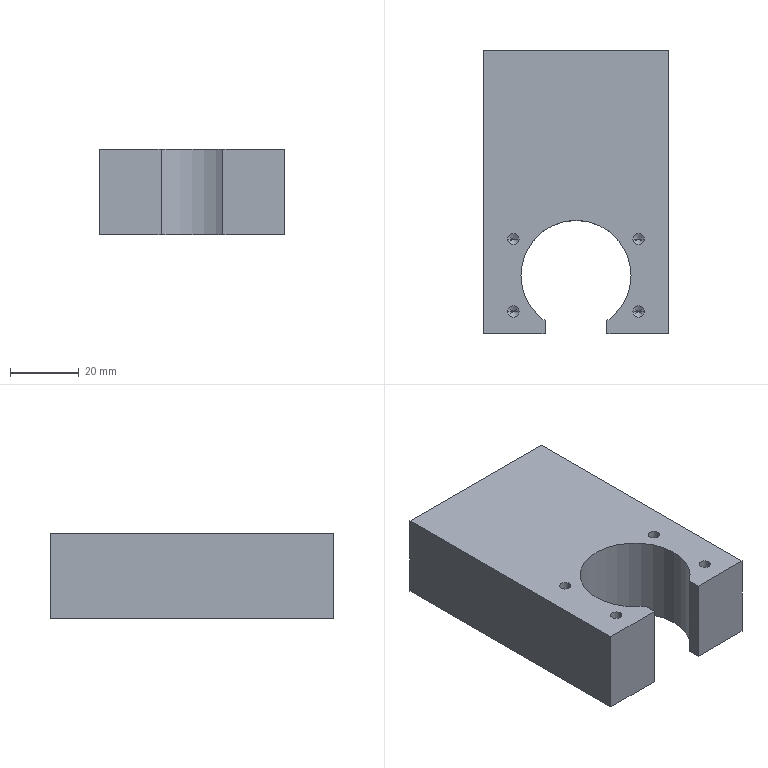Part | SolidWorks | features HoleWzd 2, 3DProfileFeature 1, Extrusion 1 | 1 solid | 52 faces | box 54 x 82.5 x 25 mm | volume 89091 mm3 | cone 24 | cylinder 19 | plane 9 | commonest cylinder face diameters 3.3 x8 5 x8 32 x3
STEP:
#1=CARTESIAN_POINT('',(-20.,64.975,3.));
#2=VERTEX_POINT('',#1);
#3=CARTESIAN_POINT('',(-20.,64.975,8.));
#4=VERTEX_POINT('',#3);
#5=CARTESIAN_POINT('',(-20.,64.975,5.5));
#6=DIRECTION('',(0.,1.,0.));
#7=DIRECTION('',(0.,0.,1.));
#8=AXIS2_PLACEMENT_3D('',#5,#6,#7);
#9=CIRCLE('',#8,2.5);
#10=EDGE_CURVE('',#2,#4,#9,.T.);
#11=ORIENTED_EDGE('',*,*,#10,.F.);
#12=CARTESIAN_POINT('',(-20.,65.5,2.475));
#13=VERTEX_POINT('',#12);
#14=CARTESIAN_POINT('',(-20.,65.5,2.475));
#15=DIRECTION('',(0.,0.7071,-0.7071));
#16=VECTOR('',#15,1000.);
#17=LINE('',#14,#16);
#18=EDGE_CURVE('',#2,#13,#17,.T.);
#19=ORIENTED_EDGE('',*,*,#18,.T.);
#20=CARTESIAN_POINT('',(-20.,65.5,8.525));
#21=VERTEX_POINT('',#20);
#22=CARTESIAN_POINT('',(-20.,65.5,5.5));
#23=DIRECTION('',(0.,1.,0.));
#24=DIRECTION('',(0.,0.,1.));
#25=AXIS2_PLACEMENT_3D('',#22,#23,#24);
#26=CIRCLE('',#25,3.025);
#27=EDGE_CURVE('',#13,#21,#26,.T.);
#28=ORIENTED_EDGE('',*,*,#27,.T.);
#29=CARTESIAN_POINT('',(-20.,65.5,8.525));
#30=DIRECTION('',(0.,0.7071,0.7071));
#31=VECTOR('',#30,1000.);
#32=LINE('',#29,#31);
#33=EDGE_CURVE('',#4,#21,#32,.T.);
#34=ORIENTED_EDGE('',*,*,#33,.F.);
#35=EDGE_LOOP('',(#11,#19,#28,#34));
#36=FACE_OUTER_BOUND('',#35,.T.);
#37=CARTESIAN_POINT('',(-20.,65.5,5.5));
#38=DIRECTION('',(0.,1.,0.));
#39=DIRECTION('',(0.,0.,1.));
#40=AXIS2_PLACEMENT_3D('',#37,#38,#39);
#41=CONICAL_SURFACE('',#40,3.025,0.7854);
#42=ADVANCED_FACE('',(#36),#41,.F.);
#43=CARTESIAN_POINT('',(-20.,53.5,3.));
#44=VERTEX_POINT('',#43);
#45=CARTESIAN_POINT('',(-20.,53.5,8.));
#46=VERTEX_POINT('',#45);
#47=CARTESIAN_POINT('',(-20.,53.5,5.5));
#48=DIRECTION('',(0.,1.,0.));
#49=DIRECTION('',(0.,0.,1.));
#50=AXIS2_PLACEMENT_3D('',#47,#48,#49);
#51=CIRCLE('',#50,2.5);
#52=EDGE_CURVE('',#44,#46,#51,.T.);
#53=ORIENTED_EDGE('',*,*,#52,.F.);
#54=CARTESIAN_POINT('',(-20.,65.5,3.));
#55=DIRECTION('',(0.,1.,0.));
#56=VECTOR('',#55,1000.);
#57=LINE('',#54,#56);
#58=EDGE_CURVE('',#44,#2,#57,.T.);
#59=ORIENTED_EDGE('',*,*,#58,.T.);
#60=ORIENTED_EDGE('',*,*,#10,.T.);
#61=CARTESIAN_POINT('',(-20.,65.5,8.));
#62=DIRECTION('',(0.,1.,0.));
#63=VECTOR('',#62,1000.);
#64=LINE('',#61,#63);
#65=EDGE_CURVE('',#46,#4,#64,.T.);
#66=ORIENTED_EDGE('',*,*,#65,.F.);
#67=EDGE_LOOP('',(#53,#59,#60,#66));
#68=FACE_OUTER_BOUND('',#67,.T.);
#69=CARTESIAN_POINT('',(-20.,65.5,5.5));
#70=DIRECTION('',(0.,1.,0.));
#71=DIRECTION('',(0.,0.,1.));
#72=AXIS2_PLACEMENT_3D('',#69,#70,#71);
#73=CYLINDRICAL_SURFACE('',#72,2.5);
#74=ADVANCED_FACE('',(#68),#73,.F.);
#75=CARTESIAN_POINT('',(-20.,51.998,5.5));
#76=VERTEX_POINT('',#75);
#77=CARTESIAN_POINT('',(-20.,53.5,8.));
#78=DIRECTION('',(0.,0.515,0.8572));
#79=VECTOR('',#78,1000.);
#80=LINE('',#77,#79);
#81=EDGE_CURVE('',#76,#46,#80,.T.);
#82=ORIENTED_EDGE('',*,*,#81,.F.);
#83=CARTESIAN_POINT('',(-20.,53.5,3.));
#84=DIRECTION('',(0.,0.515,-0.8572));
#85=VECTOR('',#84,1000.);
#86=LINE('',#83,#85);
#87=EDGE_CURVE('',#76,#44,#86,.T.);
#88=ORIENTED_EDGE('',*,*,#87,.T.);
#89=ORIENTED_EDGE('',*,*,#52,.T.);
#90=EDGE_LOOP('',(#82,#88,#89));
#91=FACE_OUTER_BOUND('',#90,.T.);
#92=CARTESIAN_POINT('',(-20.,53.5,5.5));
#93=DIRECTION('',(0.,1.,0.));
#94=DIRECTION('',(0.,0.,1.));
#95=AXIS2_PLACEMENT_3D('',#92,#93,#94);
#96=CONICAL_SURFACE('',#95,2.5,1.03);
#97=ADVANCED_FACE('',(#91),#96,.F.);
#98=CARTESIAN_POINT('',(-20.,64.975,-8.));
#99=VERTEX_POINT('',#98);
#100=CARTESIAN_POINT('',(-20.,64.975,-3.));
#101=VERTEX_POINT('',#100);
#102=CARTESIAN_POINT('',(-20.,64.975,-5.5));
#103=DIRECTION('',(0.,1.,0.));
#104=DIRECTION('',(0.,0.,1.));
#105=AXIS2_PLACEMENT_3D('',#102,#103,#104);
#106=CIRCLE('',#105,2.5);
#107=EDGE_CURVE('',#99,#101,#106,.T.);
#108=ORIENTED_EDGE('',*,*,#107,.F.);
#109=CARTESIAN_POINT('',(-20.,65.5,-8.525));
#110=VERTEX_POINT('',#109);
#111=CARTESIAN_POINT('',(-20.,65.5,-8.525));
#112=DIRECTION('',(0.,0.7071,-0.7071));
#113=VECTOR('',#112,1000.);
#114=LINE('',#111,#113);
#115=EDGE_CURVE('',#99,#110,#114,.T.);
#116=ORIENTED_EDGE('',*,*,#115,.T.);
#117=CARTESIAN_POINT('',(-20.,65.5,-2.475));
#118=VERTEX_POINT('',#117);
#119=CARTESIAN_POINT('',(-20.,65.5,-5.5));
#120=DIRECTION('',(0.,1.,0.));
#121=DIRECTION('',(0.,0.,1.));
#122=AXIS2_PLACEMENT_3D('',#119,#120,#121);
#123=CIRCLE('',#122,3.025);
#124=EDGE_CURVE('',#110,#118,#123,.T.);
#125=ORIENTED_EDGE('',*,*,#124,.T.);
#126=CARTESIAN_POINT('',(-20.,65.5,-2.475));
#127=DIRECTION('',(0.,0.7071,0.7071));
#128=VECTOR('',#127,1000.);
#129=LINE('',#126,#128);
#130=EDGE_CURVE('',#101,#118,#129,.T.);
#131=ORIENTED_EDGE('',*,*,#130,.F.);
#132=EDGE_LOOP('',(#108,#116,#125,#131));
#133=FACE_OUTER_BOUND('',#132,.T.);
#134=CARTESIAN_POINT('',(-20.,65.5,-5.5));
#135=DIRECTION('',(0.,1.,0.));
#136=DIRECTION('',(0.,0.,1.));
#137=AXIS2_PLACEMENT_3D('',#134,#135,#136);
#138=CONICAL_SURFACE('',#137,3.025,0.7854);
#139=ADVANCED_FACE('',(#133),#138,.F.);
#140=CARTESIAN_POINT('',(-20.,53.5,-8.));
#141=VERTEX_POINT('',#140);
#142=CARTESIAN_POINT('',(-20.,53.5,-3.));
#143=VERTEX_POINT('',#142);
#144=CARTESIAN_POINT('',(-20.,53.5,-5.5));
#145=DIRECTION('',(0.,1.,0.));
#146=DIRECTION('',(0.,0.,1.));
#147=AXIS2_PLACEMENT_3D('',#144,#145,#146);
#148=CIRCLE('',#147,2.5);
#149=EDGE_CURVE('',#141,#143,#148,.T.);
#150=ORIENTED_EDGE('',*,*,#149,.F.);
#151=CARTESIAN_POINT('',(-20.,65.5,-8.));
#152=DIRECTION('',(0.,1.,0.));
#153=VECTOR('',#152,1000.);
#154=LINE('',#151,#153);
#155=EDGE_CURVE('',#141,#99,#154,.T.);
#156=ORIENTED_EDGE('',*,*,#155,.T.);
#157=ORIENTED_EDGE('',*,*,#107,.T.);
#158=CARTESIAN_POINT('',(-20.,65.5,-3.));
#159=DIRECTION('',(0.,1.,0.));
#160=VECTOR('',#159,1000.);
#161=LINE('',#158,#160);
#162=EDGE_CURVE('',#143,#101,#161,.T.);
#163=ORIENTED_EDGE('',*,*,#162,.F.);
#164=EDGE_LOOP('',(#150,#156,#157,#163));
#165=FACE_OUTER_BOUND('',#164,.T.);
#166=CARTESIAN_POINT('',(-20.,65.5,-5.5));
#167=DIRECTION('',(0.,1.,0.));
#168=DIRECTION('',(0.,0.,1.));
#169=AXIS2_PLACEMENT_3D('',#166,#167,#168);
#170=CYLINDRICAL_SURFACE('',#169,2.5);
#171=ADVANCED_FACE('',(#165),#170,.F.);
#172=CARTESIAN_POINT('',(-20.,51.998,-5.5));
#173=VERTEX_POINT('',#172);
#174=CARTESIAN_POINT('',(-20.,53.5,-3.));
#175=DIRECTION('',(0.,0.515,0.8572));
#176=VECTOR('',#175,1000.);
#177=LINE('',#174,#176);
#178=EDGE_CURVE('',#173,#143,#177,.T.);
#179=ORIENTED_EDGE('',*,*,#178,.F.);
#180=CARTESIAN_POINT('',(-20.,53.5,-8.));
#181=DIRECTION('',(0.,0.515,-0.8572));
#182=VECTOR('',#181,1000.);
#183=LINE('',#180,#182);
#184=EDGE_CURVE('',#173,#141,#183,.T.);
#185=ORIENTED_EDGE('',*,*,#184,.T.);
#186=ORIENTED_EDGE('',*,*,#149,.T.);
#187=EDGE_LOOP('',(#179,#185,#186));
#188=FACE_OUTER_BOUND('',#187,.T.);
#189=CARTESIAN_POINT('',(-20.,53.5,-5.5));
#190=DIRECTION('',(0.,1.,0.));
#191=DIRECTION('',(0.,0.,1.));
#192=AXIS2_PLACEMENT_3D('',#189,#190,#191);
#193=CONICAL_SURFACE('',#192,2.5,1.03);
#194=ADVANCED_FACE('',(#188),#193,.F.);
#195=CARTESIAN_POINT('',(20.,64.975,-8.));
#196=VERTEX_POINT('',#195);
#197=CARTESIAN_POINT('',(20.,64.975,-3.));
#198=VERTEX_POINT('',#197);
#199=CARTESIAN_POINT('',(20.,64.975,-5.5));
#200=DIRECTION('',(0.,1.,0.));
#201=DIRECTION('',(0.,0.,1.));
#202=AXIS2_PLACEMENT_3D('',#199,#200,#201);
#203=CIRCLE('',#202,2.5);
#204=EDGE_CURVE('',#196,#198,#203,.T.);
#205=ORIENTED_EDGE('',*,*,#204,.F.);
#206=CARTESIAN_POINT('',(20.,65.5,-8.525));
#207=VERTEX_POINT('',#206);
#208=CARTESIAN_POINT('',(20.,65.5,-8.525));
#209=DIRECTION('',(0.,0.7071,-0.7071));
#210=VECTOR('',#209,1000.);
#211=LINE('',#208,#210);
#212=EDGE_CURVE('',#196,#207,#211,.T.);
#213=ORIENTED_EDGE('',*,*,#212,.T.);
#214=CARTESIAN_POINT('',(20.,65.5,-2.475));
#215=VERTEX_POINT('',#214);
#216=CARTESIAN_POINT('',(20.,65.5,-5.5));
#217=DIRECTION('',(0.,1.,0.));
#218=DIRECTION('',(0.,0.,1.));
#219=AXIS2_PLACEMENT_3D('',#216,#217,#218);
#220=CIRCLE('',#219,3.025);
#221=EDGE_CURVE('',#207,#215,#220,.T.);
#222=ORIENTED_EDGE('',*,*,#221,.T.);
#223=CARTESIAN_POINT('',(20.,65.5,-2.475));
#224=DIRECTION('',(0.,0.7071,0.7071));
#225=VECTOR('',#224,1000.);
#226=LINE('',#223,#225);
#227=EDGE_CURVE('',#198,#215,#226,.T.);
#228=ORIENTED_EDGE('',*,*,#227,.F.);
#229=EDGE_LOOP('',(#205,#213,#222,#228));
#230=FACE_OUTER_BOUND('',#229,.T.);
#231=CARTESIAN_POINT('',(20.,65.5,-5.5));
#232=DIRECTION('',(0.,1.,0.));
#233=DIRECTION('',(0.,0.,1.));
#234=AXIS2_PLACEMENT_3D('',#231,#232,#233);
#235=CONICAL_SURFACE('',#234,3.025,0.7854);
#236=ADVANCED_FACE('',(#230),#235,.F.);
#237=CARTESIAN_POINT('',(20.,53.5,-8.));
#238=VERTEX_POINT('',#237);
#239=CARTESIAN_POINT('',(20.,53.5,-3.));
#240=VERTEX_POINT('',#239);
#241=CARTESIAN_POINT('',(20.,53.5,-5.5));
#242=DIRECTION('',(0.,1.,0.));
#243=DIRECTION('',(0.,0.,1.));
#244=AXIS2_PLACEMENT_3D('',#241,#242,#243);
#245=CIRCLE('',#244,2.5);
#246=EDGE_CURVE('',#238,#240,#245,.T.);
#247=ORIENTED_EDGE('',*,*,#246,.F.);
#248=CARTESIAN_POINT('',(20.,65.5,-8.));
#249=DIRECTION('',(0.,1.,0.));
#250=VECTOR('',#249,1000.);
#251=LINE('',#248,#250);
#252=EDGE_CURVE('',#238,#196,#251,.T.);
#253=ORIENTED_EDGE('',*,*,#252,.T.);
#254=ORIENTED_EDGE('',*,*,#204,.T.);
#255=CARTESIAN_POINT('',(20.,65.5,-3.));
#256=DIRECTION('',(0.,1.,0.));
#257=VECTOR('',#256,1000.);
#258=LINE('',#255,#257);
#259=EDGE_CURVE('',#240,#198,#258,.T.);
#260=ORIENTED_EDGE('',*,*,#259,.F.);
#261=EDGE_LOOP('',(#247,#253,#254,#260));
#262=FACE_OUTER_BOUND('',#261,.T.);
#263=CARTESIAN_POINT('',(20.,65.5,-5.5));
#264=DIRECTION('',(0.,1.,0.));
#265=DIRECTION('',(0.,0.,1.));
#266=AXIS2_PLACEMENT_3D('',#263,#264,#265);
#267=CYLINDRICAL_SURFACE('',#266,2.5);
#268=ADVANCED_FACE('',(#262),#267,.F.);
#269=CARTESIAN_POINT('',(20.,51.998,-5.5));
#270=VERTEX_POINT('',#269);
#271=CARTESIAN_POINT('',(20.,53.5,-3.));
#272=DIRECTION('',(0.,0.515,0.8572));
#273=VECTOR('',#272,1000.);
#274=LINE('',#271,#273);
#275=EDGE_CURVE('',#270,#240,#274,.T.);
#276=ORIENTED_EDGE('',*,*,#275,.F.);
#277=CARTESIAN_POINT('',(20.,53.5,-8.));
#278=DIRECTION('',(0.,0.515,-0.8572));
#279=VECTOR('',#278,1000.);
#280=LINE('',#277,#279);
#281=EDGE_CURVE('',#270,#238,#280,.T.);
#282=ORIENTED_EDGE('',*,*,#281,.T.);
#283=ORIENTED_EDGE('',*,*,#246,.T.);
#284=EDGE_LOOP('',(#276,#282,#283));
#285=FACE_OUTER_BOUND('',#284,.T.);
#286=CARTESIAN_POINT('',(20.,53.5,-5.5));
#287=DIRECTION('',(0.,1.,0.));
#288=DIRECTION('',(0.,0.,1.));
#289=AXIS2_PLACEMENT_3D('',#286,#287,#288);
#290=CONICAL_SURFACE('',#289,2.5,1.03);
#291=ADVANCED_FACE('',(#285),#290,.F.);
#292=CARTESIAN_POINT('',(20.,64.975,3.));
#293=VERTEX_POINT('',#292);
#294=CARTESIAN_POINT('',(20.,64.975,8.));
#295=VERTEX_POINT('',#294);
#296=CARTESIAN_POINT('',(20.,64.975,5.5));
#297=DIRECTION('',(0.,1.,0.));
#298=DIRECTION('',(0.,0.,1.));
#299=AXIS2_PLACEMENT_3D('',#296,#297,#298);
#300=CIRCLE('',#299,2.5);
#301=EDGE_CURVE('',#293,#295,#300,.T.);
#302=ORIENTED_EDGE('',*,*,#301,.F.);
#303=CARTESIAN_POINT('',(20.,65.5,2.475));
#304=VERTEX_POINT('',#303);
#305=CARTESIAN_POINT('',(20.,65.5,2.475));
#306=DIRECTION('',(0.,0.7071,-0.7071));
#307=VECTOR('',#306,1000.);
#308=LINE('',#305,#307);
#309=EDGE_CURVE('',#293,#304,#308,.T.);
#310=ORIENTED_EDGE('',*,*,#309,.T.);
#311=CARTESIAN_POINT('',(20.,65.5,8.525));
#312=VERTEX_POINT('',#311);
#313=CARTESIAN_POINT('',(20.,65.5,5.5));
#314=DIRECTION('',(0.,1.,0.));
#315=DIRECTION('',(0.,0.,1.));
#316=AXIS2_PLACEMENT_3D('',#313,#314,#315);
#317=CIRCLE('',#316,3.025);
#318=EDGE_CURVE('',#304,#312,#317,.T.);
#319=ORIENTED_EDGE('',*,*,#318,.T.);
#320=CARTESIAN_POINT('',(20.,65.5,8.525));
#321=DIRECTION('',(0.,0.7071,0.7071));
#322=VECTOR('',#321,1000.);
#323=LINE('',#320,#322);
#324=EDGE_CURVE('',#295,#312,#323,.T.);
#325=ORIENTED_EDGE('',*,*,#324,.F.);
#326=EDGE_LOOP('',(#302,#310,#319,#325));
#327=FACE_OUTER_BOUND('',#326,.T.);
#328=CARTESIAN_POINT('',(20.,65.5,5.5));
#329=DIRECTION('',(0.,1.,0.));
#330=DIRECTION('',(0.,0.,1.));
#331=AXIS2_PLACEMENT_3D('',#328,#329,#330);
#332=CONICAL_SURFACE('',#331,3.025,0.7854);
#333=ADVANCED_FACE('',(#327),#332,.F.);
#334=CARTESIAN_POINT('',(20.,53.5,3.));
#335=VERTEX_POINT('',#334);
#336=CARTESIAN_POINT('',(20.,53.5,8.));
#337=VERTEX_POINT('',#336);
#338=CARTESIAN_POINT('',(20.,53.5,5.5));
#339=DIRECTION('',(0.,1.,0.));
#340=DIRECTION('',(0.,0.,1.));
#341=AXIS2_PLACEMENT_3D('',#338,#339,#340);
#342=CIRCLE('',#341,2.5);
#343=EDGE_CURVE('',#335,#337,#342,.T.);
#344=ORIENTED_EDGE('',*,*,#343,.F.);
#345=CARTESIAN_POINT('',(20.,65.5,3.));
#346=DIRECTION('',(0.,1.,0.));
#347=VECTOR('',#346,1000.);
#348=LINE('',#345,#347);
#349=EDGE_CURVE('',#335,#293,#348,.T.);
#350=ORIENTED_EDGE('',*,*,#349,.T.);
#351=ORIENTED_EDGE('',*,*,#301,.T.);
#352=CARTESIAN_POINT('',(20.,65.5,8.));
#353=DIRECTION('',(0.,1.,0.));
#354=VECTOR('',#353,1000.);
#355=LINE('',#352,#354);
#356=EDGE_CURVE('',#337,#295,#355,.T.);
#357=ORIENTED_EDGE('',*,*,#356,.F.);
#358=EDGE_LOOP('',(#344,#350,#351,#357));
#359=FACE_OUTER_BOUND('',#358,.T.);
#360=CARTESIAN_POINT('',(20.,65.5,5.5));
#361=DIRECTION('',(0.,1.,0.));
#362=DIRECTION('',(0.,0.,1.));
#363=AXIS2_PLACEMENT_3D('',#360,#361,#362);
#364=CYLINDRICAL_SURFACE('',#363,2.5);
#365=ADVANCED_FACE('',(#359),#364,.F.);
#366=CARTESIAN_POINT('',(20.,51.998,5.5));
#367=VERTEX_POINT('',#366);
#368=CARTESIAN_POINT('',(20.,53.5,8.));
#369=DIRECTION('',(0.,0.515,0.8572));
#370=VECTOR('',#369,1000.);
#371=LINE('',#368,#370);
#372=EDGE_CURVE('',#367,#337,#371,.T.);
#373=ORIENTED_EDGE('',*,*,#372,.F.);
#374=CARTESIAN_POINT('',(20.,53.5,3.));
#375=DIRECTION('',(0.,0.515,-0.8572));
#376=VECTOR('',#375,1000.);
#377=LINE('',#374,#376);
#378=EDGE_CURVE('',#367,#335,#377,.T.);
#379=ORIENTED_EDGE('',*,*,#378,.T.);
#380=ORIENTED_EDGE('',*,*,#343,.T.);
#381=EDGE_LOOP('',(#373,#379,#380));
#382=FACE_OUTER_BOUND('',#381,.T.);
#383=CARTESIAN_POINT('',(20.,53.5,5.5));
#384=DIRECTION('',(0.,1.,0.));
#385=DIRECTION('',(0.,0.,1.));
#386=AXIS2_PLACEMENT_3D('',#383,#384,#385);
#387=CONICAL_SURFACE('',#386,2.5,1.03);
#388=ADVANCED_FACE('',(#382),#387,.F.);
#389=CARTESIAN_POINT('',(16.537,10.5,3.));
#390=VERTEX_POINT('',#389);
#391=CARTESIAN_POINT('',(19.837,10.5,3.));
#392=VERTEX_POINT('',#391);
#393=CARTESIAN_POINT('',(18.187,10.5,3.));
#394=DIRECTION('',(0.,0.,1.));
#395=DIRECTION('',(1.,0.,0.));
#396=AXIS2_PLACEMENT_3D('',#393,#394,#395);
#397=CIRCLE('',#396,1.65);
#398=EDGE_CURVE('',#390,#392,#397,.T.);
#399=ORIENTED_EDGE('',*,*,#398,.F.);
#400=CARTESIAN_POINT('',(16.537,10.5,12.5));
#401=VERTEX_POINT('',#400);
#402=CARTESIAN_POINT('',(16.537,10.5,12.5));
#403=DIRECTION('',(0.,0.,1.));
#404=VECTOR('',#403,1000.);
#405=LINE('',#402,#404);
#406=EDGE_CURVE('',#390,#401,#405,.T.);
#407=ORIENTED_EDGE('',*,*,#406,.T.);
#408=CARTESIAN_POINT('',(19.837,10.5,12.5));
#409=VERTEX_POINT('',#408);
#410=CARTESIAN_POINT('',(18.187,10.5,12.5));
#411=DIRECTION('',(0.,0.,1.));
#412=DIRECTION('',(1.,0.,0.));
#413=AXIS2_PLACEMENT_3D('',#410,#411,#412);
#414=CIRCLE('',#413,1.65);
#415=EDGE_CURVE('',#401,#409,#414,.T.);
#416=ORIENTED_EDGE('',*,*,#415,.T.);
#417=CARTESIAN_POINT('',(19.837,10.5,12.5));
#418=DIRECTION('',(0.,0.,1.));
#419=VECTOR('',#418,1000.);
#420=LINE('',#417,#419);
#421=EDGE_CURVE('',#392,#409,#420,.T.);
#422=ORIENTED_EDGE('',*,*,#421,.F.);
#423=EDGE_LOOP('',(#399,#407,#416,#422));
#424=FACE_OUTER_BOUND('',#423,.T.);
#425=CARTESIAN_POINT('',(18.187,10.5,12.5));
#426=DIRECTION('',(0.,0.,1.));
#427=DIRECTION('',(1.,0.,0.));
#428=AXIS2_PLACEMENT_3D('',#425,#426,#427);
#429=CYLINDRICAL_SURFACE('',#428,1.65);
#430=ADVANCED_FACE('',(#424),#429,.F.);
#431=CARTESIAN_POINT('',(18.187,10.5,2.009));
#432=VERTEX_POINT('',#431);
#433=CARTESIAN_POINT('',(19.837,10.5,3.));
#434=DIRECTION('',(0.8572,0.,0.515));
#435=VECTOR('',#434,1000.);
#436=LINE('',#433,#435);
#437=EDGE_CURVE('',#432,#392,#436,.T.);
#438=ORIENTED_EDGE('',*,*,#437,.F.);
#439=CARTESIAN_POINT('',(16.537,10.5,3.));
#440=DIRECTION('',(-0.8572,0.,0.515));
#441=VECTOR('',#440,1000.);
#442=LINE('',#439,#441);
#443=EDGE_CURVE('',#432,#390,#442,.T.);
#444=ORIENTED_EDGE('',*,*,#443,.T.);
#445=ORIENTED_EDGE('',*,*,#398,.T.);
#446=EDGE_LOOP('',(#438,#444,#445));
#447=FACE_OUTER_BOUND('',#446,.T.);
#448=CARTESIAN_POINT('',(18.187,10.5,3.));
#449=DIRECTION('',(0.,0.,1.));
#450=DIRECTION('',(1.,0.,0.));
#451=AXIS2_PLACEMENT_3D('',#448,#449,#450);
#452=CONICAL_SURFACE('',#451,1.65,1.03);
#453=ADVANCED_FACE('',(#447),#452,.F.);
#454=CARTESIAN_POINT('',(16.537,-10.5,3.));
#455=VERTEX_POINT('',#454);
#456=CARTESIAN_POINT('',(19.837,-10.5,3.));
#457=VERTEX_POINT('',#456);
#458=CARTESIAN_POINT('',(18.187,-10.5,3.));
#459=DIRECTION('',(0.,0.,1.));
#460=DIRECTION('',(1.,0.,0.));
#461=AXIS2_PLACEMENT_3D('',#458,#459,#460);
#462=CIRCLE('',#461,1.65);
#463=EDGE_CURVE('',#455,#457,#462,.T.);
#464=ORIENTED_EDGE('',*,*,#463,.F.);
#465=CARTESIAN_POINT('',(16.537,-10.5,12.5));
#466=VERTEX_POINT('',#465);
#467=CARTESIAN_POINT('',(16.537,-10.5,12.5));
#468=DIRECTION('',(0.,0.,1.));
#469=VECTOR('',#468,1000.);
#470=LINE('',#467,#469);
#471=EDGE_CURVE('',#455,#466,#470,.T.);
#472=ORIENTED_EDGE('',*,*,#471,.T.);
#473=CARTESIAN_POINT('',(19.837,-10.5,12.5));
#474=VERTEX_POINT('',#473);
#475=CARTESIAN_POINT('',(18.187,-10.5,12.5));
#476=DIRECTION('',(0.,0.,1.));
#477=DIRECTION('',(1.,0.,0.));
#478=AXIS2_PLACEMENT_3D('',#475,#476,#477);
#479=CIRCLE('',#478,1.65);
#480=EDGE_CURVE('',#466,#474,#479,.T.);
#481=ORIENTED_EDGE('',*,*,#480,.T.);
#482=CARTESIAN_POINT('',(19.837,-10.5,12.5));
#483=DIRECTION('',(0.,0.,1.));
#484=VECTOR('',#483,1000.);
#485=LINE('',#482,#484);
#486=EDGE_CURVE('',#457,#474,#485,.T.);
#487=ORIENTED_EDGE('',*,*,#486,.F.);
#488=EDGE_LOOP('',(#464,#472,#481,#487));
#489=FACE_OUTER_BOUND('',#488,.T.);
#490=CARTESIAN_POINT('',(18.187,-10.5,12.5));
#491=DIRECTION('',(0.,0.,1.));
#492=DIRECTION('',(1.,0.,0.));
#493=AXIS2_PLACEMENT_3D('',#490,#491,#492);
#494=CYLINDRICAL_SURFACE('',#493,1.65);
#495=ADVANCED_FACE('',(#489),#494,.F.);
#496=CARTESIAN_POINT('',(18.187,-10.5,2.009));
#497=VERTEX_POINT('',#496);
#498=CARTESIAN_POINT('',(19.837,-10.5,3.));
#499=DIRECTION('',(0.8572,0.,0.515));
#500=VECTOR('',#499,1000.);
#501=LINE('',#498,#500);
#502=EDGE_CURVE('',#497,#457,#501,.T.);
#503=ORIENTED_EDGE('',*,*,#502,.F.);
#504=CARTESIAN_POINT('',(16.537,-10.5,3.));
#505=DIRECTION('',(-0.8572,0.,0.515));
#506=VECTOR('',#505,1000.);
#507=LINE('',#504,#506);
#508=EDGE_CURVE('',#497,#455,#507,.T.);
#509=ORIENTED_EDGE('',*,*,#508,.T.);
#510=ORIENTED_EDGE('',*,*,#463,.T.);
#511=EDGE_LOOP('',(#503,#509,#510));
#512=FACE_OUTER_BOUND('',#511,.T.);
#513=CARTESIAN_POINT('',(18.187,-10.5,3.));
#514=DIRECTION('',(0.,0.,1.));
#515=DIRECTION('',(1.,0.,0.));
#516=AXIS2_PLACEMENT_3D('',#513,#514,#515);
#517=CONICAL_SURFACE('',#516,1.65,1.03);
#518=ADVANCED_FACE('',(#512),#517,.F.);
#519=CARTESIAN_POINT('',(-19.837,-10.5,3.));
#520=VERTEX_POINT('',#519);
#521=CARTESIAN_POINT('',(-16.537,-10.5,3.));
#522=VERTEX_POINT('',#521);
#523=CARTESIAN_POINT('',(-18.187,-10.5,3.));
#524=DIRECTION('',(0.,0.,1.));
#525=DIRECTION('',(1.,0.,0.));
#526=AXIS2_PLACEMENT_3D('',#523,#524,#525);
#527=CIRCLE('',#526,1.65);
#528=EDGE_CURVE('',#520,#522,#527,.T.);
#529=ORIENTED_EDGE('',*,*,#528,.F.);
#530=CARTESIAN_POINT('',(-19.837,-10.5,12.5));
#531=VERTEX_POINT('',#530);
#532=CARTESIAN_POINT('',(-19.837,-10.5,12.5));
#533=DIRECTION('',(0.,0.,1.));
#534=VECTOR('',#533,1000.);
#535=LINE('',#532,#534);
#536=EDGE_CURVE('',#520,#531,#535,.T.);
#537=ORIENTED_EDGE('',*,*,#536,.T.);
#538=CARTESIAN_POINT('',(-16.537,-10.5,12.5));
#539=VERTEX_POINT('',#538);
#540=CARTESIAN_POINT('',(-18.187,-10.5,12.5));
#541=DIRECTION('',(0.,0.,1.));
#542=DIRECTION('',(1.,0.,0.));
#543=AXIS2_PLACEMENT_3D('',#540,#541,#542);
#544=CIRCLE('',#543,1.65);
#545=EDGE_CURVE('',#531,#539,#544,.T.);
#546=ORIENTED_EDGE('',*,*,#545,.T.);
#547=CARTESIAN_POINT('',(-16.537,-10.5,12.5));
#548=DIRECTION('',(0.,0.,1.));
#549=VECTOR('',#548,1000.);
#550=LINE('',#547,#549);
#551=EDGE_CURVE('',#522,#539,#550,.T.);
#552=ORIENTED_EDGE('',*,*,#551,.F.);
#553=EDGE_LOOP('',(#529,#537,#546,#552));
#554=FACE_OUTER_BOUND('',#553,.T.);
#555=CARTESIAN_POINT('',(-18.187,-10.5,12.5));
#556=DIRECTION('',(0.,0.,1.));
#557=DIRECTION('',(1.,0.,0.));
#558=AXIS2_PLACEMENT_3D('',#555,#556,#557);
#559=CYLINDRICAL_SURFACE('',#558,1.65);
#560=ADVANCED_FACE('',(#554),#559,.F.);
#561=CARTESIAN_POINT('',(-18.187,-10.5,2.009));
#562=VERTEX_POINT('',#561);
#563=CARTESIAN_POINT('',(-16.537,-10.5,3.));
#564=DIRECTION('',(0.8572,0.,0.515));
#565=VECTOR('',#564,1000.);
#566=LINE('',#563,#565);
#567=EDGE_CURVE('',#562,#522,#566,.T.);
#568=ORIENTED_EDGE('',*,*,#567,.F.);
#569=CARTESIAN_POINT('',(-19.837,-10.5,3.));
#570=DIRECTION('',(-0.8572,0.,0.515));
#571=VECTOR('',#570,1000.);
#572=LINE('',#569,#571);
#573=EDGE_CURVE('',#562,#520,#572,.T.);
#574=ORIENTED_EDGE('',*,*,#573,.T.);
#575=ORIENTED_EDGE('',*,*,#528,.T.);
#576=EDGE_LOOP('',(#568,#574,#575));
#577=FACE_OUTER_BOUND('',#576,.T.);
#578=CARTESIAN_POINT('',(-18.187,-10.5,3.));
#579=DIRECTION('',(0.,0.,1.));
#580=DIRECTION('',(1.,0.,0.));
#581=AXIS2_PLACEMENT_3D('',#578,#579,#580);
#582=CONICAL_SURFACE('',#581,1.65,1.03);
#583=ADVANCED_FACE('',(#577),#582,.F.);
#584=CARTESIAN_POINT('',(-19.837,10.5,3.));
#585=VERTEX_POINT('',#584);
#586=CARTESIAN_POINT('',(-16.537,10.5,3.));
#587=VERTEX_POINT('',#586);
#588=CARTESIAN_POINT('',(-18.187,10.5,3.));
#589=DIRECTION('',(0.,0.,1.));
#590=DIRECTION('',(1.,0.,0.));
#591=AXIS2_PLACEMENT_3D('',#588,#589,#590);
#592=CIRCLE('',#591,1.65);
#593=EDGE_CURVE('',#585,#587,#592,.T.);
#594=ORIENTED_EDGE('',*,*,#593,.F.);
#595=CARTESIAN_POINT('',(-19.837,10.5,12.5));
#596=VERTEX_POINT('',#595);
#597=CARTESIAN_POINT('',(-19.837,10.5,12.5));
#598=DIRECTION('',(0.,0.,1.));
#599=VECTOR('',#598,1000.);
#600=LINE('',#597,#599);
#601=EDGE_CURVE('',#585,#596,#600,.T.);
#602=ORIENTED_EDGE('',*,*,#601,.T.);
#603=CARTESIAN_POINT('',(-16.537,10.5,12.5));
#604=VERTEX_POINT('',#603);
#605=CARTESIAN_POINT('',(-18.187,10.5,12.5));
#606=DIRECTION('',(0.,0.,1.));
#607=DIRECTION('',(1.,0.,0.));
#608=AXIS2_PLACEMENT_3D('',#605,#606,#607);
#609=CIRCLE('',#608,1.65);
#610=EDGE_CURVE('',#596,#604,#609,.T.);
#611=ORIENTED_EDGE('',*,*,#610,.T.);
#612=CARTESIAN_POINT('',(-16.537,10.5,12.5));
#613=DIRECTION('',(0.,0.,1.));
#614=VECTOR('',#613,1000.);
#615=LINE('',#612,#614);
#616=EDGE_CURVE('',#587,#604,#615,.T.);
#617=ORIENTED_EDGE('',*,*,#616,.F.);
#618=EDGE_LOOP('',(#594,#602,#611,#617));
#619=FACE_OUTER_BOUND('',#618,.T.);
#620=CARTESIAN_POINT('',(-18.187,10.5,12.5));
#621=DIRECTION('',(0.,0.,1.));
#622=DIRECTION('',(1.,0.,0.));
#623=AXIS2_PLACEMENT_3D('',#620,#621,#622);
#624=CYLINDRICAL_SURFACE('',#623,1.65);
#625=ADVANCED_FACE('',(#619),#624,.F.);
#626=CARTESIAN_POINT('',(-18.187,10.5,2.009));
#627=VERTEX_POINT('',#626);
#628=CARTESIAN_POINT('',(-16.537,10.5,3.));
#629=DIRECTION('',(0.8572,0.,0.515));
#630=VECTOR('',#629,1000.);
#631=LINE('',#628,#630);
#632=EDGE_CURVE('',#627,#587,#631,.T.);
#633=ORIENTED_EDGE('',*,*,#632,.F.);
#634=CARTESIAN_POINT('',(-19.837,10.5,3.));
#635=DIRECTION('',(-0.8572,0.,0.515));
#636=VECTOR('',#635,1000.);
#637=LINE('',#634,#636);
#638=EDGE_CURVE('',#627,#585,#637,.T.);
#639=ORIENTED_EDGE('',*,*,#638,.T.);
#640=ORIENTED_EDGE('',*,*,#593,.T.);
#641=EDGE_LOOP('',(#633,#639,#640));
#642=FACE_OUTER_BOUND('',#641,.T.);
#643=CARTESIAN_POINT('',(-18.187,10.5,3.));
#644=DIRECTION('',(0.,0.,1.));
#645=DIRECTION('',(1.,0.,0.));
#646=AXIS2_PLACEMENT_3D('',#643,#644,#645);
#647=CONICAL_SURFACE('',#646,1.65,1.03);
#648=ADVANCED_FACE('',(#642),#647,.F.);
#649=CARTESIAN_POINT('',(16.,0.,12.5));
#650=VERTEX_POINT('',#649);
#651=CARTESIAN_POINT('',(9.,-13.229,12.5));
#652=VERTEX_POINT('',#651);
#653=CARTESIAN_POINT('',(0.,0.,12.5));
#654=DIRECTION('',(0.,0.,-1.));
#655=DIRECTION('',(1.,0.,0.));
#656=AXIS2_PLACEMENT_3D('',#653,#654,#655);
#657=CIRCLE('',#656,16.);
#658=EDGE_CURVE('',#650,#652,#657,.T.);
#659=ORIENTED_EDGE('',*,*,#658,.F.);
#660=CARTESIAN_POINT('',(16.,0.,-12.5));
#661=VERTEX_POINT('',#660);
#662=CARTESIAN_POINT('',(16.,0.,12.5));
#663=DIRECTION('',(0.,0.,-1.));
#664=VECTOR('',#663,1000.);
#665=LINE('',#662,#664);
#666=EDGE_CURVE('',#650,#661,#665,.T.);
#667=ORIENTED_EDGE('',*,*,#666,.T.);
#668=CARTESIAN_POINT('',(9.,-13.229,-12.5));
#669=VERTEX_POINT('',#668);
#670=CARTESIAN_POINT('',(0.,0.,-12.5));
#671=DIRECTION('',(0.,0.,-1.));
#672=DIRECTION('',(1.,0.,0.));
#673=AXIS2_PLACEMENT_3D('',#670,#671,#672);
#674=CIRCLE('',#673,16.);
#675=EDGE_CURVE('',#661,#669,#674,.T.);
#676=ORIENTED_EDGE('',*,*,#675,.T.);
#677=CARTESIAN_POINT('',(9.,-13.229,12.5));
#678=DIRECTION('',(0.,0.,-1.));
#679=VECTOR('',#678,1000.);
#680=LINE('',#677,#679);
#681=EDGE_CURVE('',#652,#669,#680,.T.);
#682=ORIENTED_EDGE('',*,*,#681,.F.);
#683=EDGE_LOOP('',(#659,#667,#676,#682));
#684=FACE_OUTER_BOUND('',#683,.T.);
#685=CARTESIAN_POINT('',(0.,0.,12.5));
#686=DIRECTION('',(0.,0.,-1.));
#687=DIRECTION('',(-1.,0.,0.));
#688=AXIS2_PLACEMENT_3D('',#685,#686,#687);
#689=CYLINDRICAL_SURFACE('',#688,16.);
#690=ADVANCED_FACE('',(#684),#689,.F.);
#691=ORIENTED_EDGE('',*,*,#666,.F.);
#692=CARTESIAN_POINT('',(-16.,0.,12.5));
#693=VERTEX_POINT('',#692);
#694=CARTESIAN_POINT('',(0.,0.,12.5));
#695=DIRECTION('',(0.,0.,-1.));
#696=DIRECTION('',(1.,0.,0.));
#697=AXIS2_PLACEMENT_3D('',#694,#695,#696);
#698=CIRCLE('',#697,16.);
#699=EDGE_CURVE('',#693,#650,#698,.T.);
#700=ORIENTED_EDGE('',*,*,#699,.F.);
#701=CARTESIAN_POINT('',(-16.,0.,-12.5));
#702=VERTEX_POINT('',#701);
#703=CARTESIAN_POINT('',(-16.,0.,12.5));
#704=DIRECTION('',(0.,0.,-1.));
#705=VECTOR('',#704,1000.);
#706=LINE('',#703,#705);
#707=EDGE_CURVE('',#693,#702,#706,.T.);
#708=ORIENTED_EDGE('',*,*,#707,.T.);
#709=CARTESIAN_POINT('',(0.,0.,-12.5));
#710=DIRECTION('',(0.,0.,-1.));
#711=DIRECTION('',(1.,0.,0.));
#712=AXIS2_PLACEMENT_3D('',#709,#710,#711);
#713=CIRCLE('',#712,16.);
#714=EDGE_CURVE('',#702,#661,#713,.T.);
#715=ORIENTED_EDGE('',*,*,#714,.T.);
#716=EDGE_LOOP('',(#691,#700,#708,#715));
#717=FACE_OUTER_BOUND('',#716,.T.);
#718=CARTESIAN_POINT('',(0.,0.,12.5));
#719=DIRECTION('',(0.,0.,-1.));
#720=DIRECTION('',(-1.,0.,0.));
#721=AXIS2_PLACEMENT_3D('',#718,#719,#720);
#722=CYLINDRICAL_SURFACE('',#721,16.);
#723=ADVANCED_FACE('',(#717),#722,.F.);
#724=CARTESIAN_POINT('',(-27.,65.5,-12.5));
#725=VERTEX_POINT('',#724);
#726=CARTESIAN_POINT('',(-27.,-17.,-12.5));
#727=VERTEX_POINT('',#726);
#728=CARTESIAN_POINT('',(-27.,65.5,-12.5));
#729=DIRECTION('',(0.,-1.,0.));
#730=VECTOR('',#729,1000.);
#731=LINE('',#728,#730);
#732=EDGE_CURVE('',#725,#727,#731,.T.);
#733=ORIENTED_EDGE('',*,*,#732,.T.);
#734=CARTESIAN_POINT('',(-27.,-17.,12.5));
#735=VERTEX_POINT('',#734);
#736=CARTESIAN_POINT('',(-27.,-17.,12.5));
#737=DIRECTION('',(0.,0.,-1.));
#738=VECTOR('',#737,1000.);
#739=LINE('',#736,#738);
#740=EDGE_CURVE('',#735,#727,#739,.T.);
#741=ORIENTED_EDGE('',*,*,#740,.F.);
#742=CARTESIAN_POINT('',(-27.,65.5,12.5));
#743=VERTEX_POINT('',#742);
#744=CARTESIAN_POINT('',(-27.,65.5,12.5));
#745=DIRECTION('',(0.,-1.,0.));
#746=VECTOR('',#745,1000.);
#747=LINE('',#744,#746);
#748=EDGE_CURVE('',#743,#735,#747,.T.);
#749=ORIENTED_EDGE('',*,*,#748,.F.);
#750=CARTESIAN_POINT('',(-27.,65.5,12.5));
#751=DIRECTION('',(0.,0.,-1.));
#752=VECTOR('',#751,1000.);
#753=LINE('',#750,#752);
#754=EDGE_CURVE('',#743,#725,#753,.T.);
#755=ORIENTED_EDGE('',*,*,#754,.T.);
#756=EDGE_LOOP('',(#733,#741,#749,#755));
#757=FACE_OUTER_BOUND('',#756,.T.);
#758=CARTESIAN_POINT('',(-27.,65.5,12.5));
#759=DIRECTION('',(1.,0.,0.));
#760=DIRECTION('',(0.,1.,0.));
#761=AXIS2_PLACEMENT_3D('',#758,#759,#760);
#762=PLANE('',#761);
#763=ADVANCED_FACE('',(#757),#762,.F.);
#764=CARTESIAN_POINT('',(-9.,-17.,-12.5));
#765=VERTEX_POINT('',#764);
#766=CARTESIAN_POINT('',(-27.,-17.,-12.5));
#767=DIRECTION('',(1.,0.,0.));
#768=VECTOR('',#767,1000.);
#769=LINE('',#766,#768);
#770=EDGE_CURVE('',#727,#765,#769,.T.);
#771=ORIENTED_EDGE('',*,*,#770,.T.);
#772=CARTESIAN_POINT('',(-9.,-17.,12.5));
#773=VERTEX_POINT('',#772);
#774=CARTESIAN_POINT('',(-9.,-17.,12.5));
#775=DIRECTION('',(0.,0.,-1.));
#776=VECTOR('',#775,1000.);
#777=LINE('',#774,#776);
#778=EDGE_CURVE('',#773,#765,#777,.T.);
#779=ORIENTED_EDGE('',*,*,#778,.F.);
#780=CARTESIAN_POINT('',(-27.,-17.,12.5));
#781=DIRECTION('',(1.,0.,0.));
#782=VECTOR('',#781,1000.);
#783=LINE('',#780,#782);
#784=EDGE_CURVE('',#735,#773,#783,.T.);
#785=ORIENTED_EDGE('',*,*,#784,.F.);
#786=ORIENTED_EDGE('',*,*,#740,.T.);
#787=EDGE_LOOP('',(#771,#779,#785,#786));
#788=FACE_OUTER_BOUND('',#787,.T.);
#789=CARTESIAN_POINT('',(-27.,-17.,12.5));
#790=DIRECTION('',(0.,1.,0.));
#791=DIRECTION('',(0.,0.,1.));
#792=AXIS2_PLACEMENT_3D('',#789,#790,#791);
#793=PLANE('',#792);
#794=ADVANCED_FACE('',(#788),#793,.F.);
#795=CARTESIAN_POINT('',(-9.,-13.229,-12.5));
#796=VERTEX_POINT('',#795);
#797=CARTESIAN_POINT('',(-9.,-17.,-12.5));
#798=DIRECTION('',(0.,1.,0.));
#799=VECTOR('',#798,1000.);
#800=LINE('',#797,#799);
#801=EDGE_CURVE('',#765,#796,#800,.T.);
#802=ORIENTED_EDGE('',*,*,#801,.T.);
#803=CARTESIAN_POINT('',(-9.,-13.229,12.5));
#804=VERTEX_POINT('',#803);
#805=CARTESIAN_POINT('',(-9.,-13.229,12.5));
#806=DIRECTION('',(0.,0.,-1.));
#807=VECTOR('',#806,1000.);
#808=LINE('',#805,#807);
#809=EDGE_CURVE('',#804,#796,#808,.T.);
#810=ORIENTED_EDGE('',*,*,#809,.F.);
#811=CARTESIAN_POINT('',(-9.,-17.,12.5));
#812=DIRECTION('',(0.,1.,0.));
#813=VECTOR('',#812,1000.);
#814=LINE('',#811,#813);
#815=EDGE_CURVE('',#773,#804,#814,.T.);
#816=ORIENTED_EDGE('',*,*,#815,.F.);
#817=ORIENTED_EDGE('',*,*,#778,.T.);
#818=EDGE_LOOP('',(#802,#810,#816,#817));
#819=FACE_OUTER_BOUND('',#818,.T.);
#820=CARTESIAN_POINT('',(-9.,-17.,12.5));
#821=DIRECTION('',(-1.,0.,0.));
#822=DIRECTION('',(0.,-1.,0.));
#823=AXIS2_PLACEMENT_3D('',#820,#821,#822);
#824=PLANE('',#823);
#825=ADVANCED_FACE('',(#819),#824,.F.);
#826=ORIENTED_EDGE('',*,*,#707,.F.);
#827=CARTESIAN_POINT('',(0.,0.,12.5));
#828=DIRECTION('',(0.,0.,-1.));
#829=DIRECTION('',(1.,0.,0.));
#830=AXIS2_PLACEMENT_3D('',#827,#828,#829);
#831=CIRCLE('',#830,16.);
#832=EDGE_CURVE('',#804,#693,#831,.T.);
#833=ORIENTED_EDGE('',*,*,#832,.F.);
#834=ORIENTED_EDGE('',*,*,#809,.T.);
#835=CARTESIAN_POINT('',(0.,0.,-12.5));
#836=DIRECTION('',(0.,0.,-1.));
#837=DIRECTION('',(1.,0.,0.));
#838=AXIS2_PLACEMENT_3D('',#835,#836,#837);
#839=CIRCLE('',#838,16.);
#840=EDGE_CURVE('',#796,#702,#839,.T.);
#841=ORIENTED_EDGE('',*,*,#840,.T.);
#842=EDGE_LOOP('',(#826,#833,#834,#841));
#843=FACE_OUTER_BOUND('',#842,.T.);
#844=CARTESIAN_POINT('',(0.,0.,12.5));
#845=DIRECTION('',(0.,0.,-1.));
#846=DIRECTION('',(-1.,0.,0.));
#847=AXIS2_PLACEMENT_3D('',#844,#845,#846);
#848=CYLINDRICAL_SURFACE('',#847,16.);
#849=ADVANCED_FACE('',(#843),#848,.F.);
#850=CARTESIAN_POINT('',(9.,-17.,-12.5));
#851=VERTEX_POINT('',#850);
#852=CARTESIAN_POINT('',(9.,-17.,-12.5));
#853=DIRECTION('',(0.,-1.,0.));
#854=VECTOR('',#853,1000.);
#855=LINE('',#852,#854);
#856=EDGE_CURVE('',#669,#851,#855,.T.);
#857=ORIENTED_EDGE('',*,*,#856,.T.);
#858=CARTESIAN_POINT('',(9.,-17.,12.5));
#859=VERTEX_POINT('',#858);
#860=CARTESIAN_POINT('',(9.,-17.,12.5));
#861=DIRECTION('',(0.,0.,-1.));
#862=VECTOR('',#861,1000.);
#863=LINE('',#860,#862);
#864=EDGE_CURVE('',#859,#851,#863,.T.);
#865=ORIENTED_EDGE('',*,*,#864,.F.);
#866=CARTESIAN_POINT('',(9.,-17.,12.5));
#867=DIRECTION('',(0.,-1.,0.));
#868=VECTOR('',#867,1000.);
#869=LINE('',#866,#868);
#870=EDGE_CURVE('',#652,#859,#869,.T.);
#871=ORIENTED_EDGE('',*,*,#870,.F.);
#872=ORIENTED_EDGE('',*,*,#681,.T.);
#873=EDGE_LOOP('',(#857,#865,#871,#872));
#874=FACE_OUTER_BOUND('',#873,.T.);
#875=CARTESIAN_POINT('',(9.,-17.,12.5));
#876=DIRECTION('',(1.,0.,0.));
#877=DIRECTION('',(0.,0.,-1.));
#878=AXIS2_PLACEMENT_3D('',#875,#876,#877);
#879=PLANE('',#878);
#880=ADVANCED_FACE('',(#874),#879,.F.);
#881=CARTESIAN_POINT('',(27.,-17.,-12.5));
#882=VERTEX_POINT('',#881);
#883=CARTESIAN_POINT('',(27.,-17.,-12.5));
#884=DIRECTION('',(1.,0.,0.));
#885=VECTOR('',#884,1000.);
#886=LINE('',#883,#885);
#887=EDGE_CURVE('',#851,#882,#886,.T.);
#888=ORIENTED_EDGE('',*,*,#887,.T.);
#889=CARTESIAN_POINT('',(27.,-17.,12.5));
#890=VERTEX_POINT('',#889);
#891=CARTESIAN_POINT('',(27.,-17.,12.5));
#892=DIRECTION('',(0.,0.,-1.));
#893=VECTOR('',#892,1000.);
#894=LINE('',#891,#893);
#895=EDGE_CURVE('',#890,#882,#894,.T.);
#896=ORIENTED_EDGE('',*,*,#895,.F.);
#897=CARTESIAN_POINT('',(27.,-17.,12.5));
#898=DIRECTION('',(1.,0.,0.));
#899=VECTOR('',#898,1000.);
#900=LINE('',#897,#899);
#901=EDGE_CURVE('',#859,#890,#900,.T.);
#902=ORIENTED_EDGE('',*,*,#901,.F.);
#903=ORIENTED_EDGE('',*,*,#864,.T.);
#904=EDGE_LOOP('',(#888,#896,#902,#903));
#905=FACE_OUTER_BOUND('',#904,.T.);
#906=CARTESIAN_POINT('',(27.,-17.,12.5));
#907=DIRECTION('',(0.,1.,0.));
#908=DIRECTION('',(-1.,0.,0.));
#909=AXIS2_PLACEMENT_3D('',#906,#907,#908);
#910=PLANE('',#909);
#911=ADVANCED_FACE('',(#905),#910,.F.);
#912=CARTESIAN_POINT('',(27.,65.5,-12.5));
#913=VERTEX_POINT('',#912);
#914=CARTESIAN_POINT('',(27.,65.5,-12.5));
#915=DIRECTION('',(0.,1.,0.));
#916=VECTOR('',#915,1000.);
#917=LINE('',#914,#916);
#918=EDGE_CURVE('',#882,#913,#917,.T.);
#919=ORIENTED_EDGE('',*,*,#918,.T.);
#920=CARTESIAN_POINT('',(27.,65.5,12.5));
#921=VERTEX_POINT('',#920);
#922=CARTESIAN_POINT('',(27.,65.5,12.5));
#923=DIRECTION('',(0.,0.,-1.));
#924=VECTOR('',#923,1000.);
#925=LINE('',#922,#924);
#926=EDGE_CURVE('',#921,#913,#925,.T.);
#927=ORIENTED_EDGE('',*,*,#926,.F.);
#928=CARTESIAN_POINT('',(27.,65.5,12.5));
#929=DIRECTION('',(0.,1.,0.));
#930=VECTOR('',#929,1000.);
#931=LINE('',#928,#930);
#932=EDGE_CURVE('',#890,#921,#931,.T.);
#933=ORIENTED_EDGE('',*,*,#932,.F.);
#934=ORIENTED_EDGE('',*,*,#895,.T.);
#935=EDGE_LOOP('',(#919,#927,#933,#934));
#936=FACE_OUTER_BOUND('',#935,.T.);
#937=CARTESIAN_POINT('',(27.,65.5,12.5));
#938=DIRECTION('',(-1.,0.,0.));
#939=DIRECTION('',(0.,-1.,0.));
#940=AXIS2_PLACEMENT_3D('',#937,#938,#939);
#941=PLANE('',#940);
#942=ADVANCED_FACE('',(#936),#941,.F.);
#943=CARTESIAN_POINT('',(-20.,65.5,5.5));
#944=DIRECTION('',(0.,1.,0.));
#945=DIRECTION('',(0.,0.,1.));
#946=AXIS2_PLACEMENT_3D('',#943,#944,#945);
#947=CIRCLE('',#946,3.025);
#948=EDGE_CURVE('',#21,#13,#947,.T.);
#949=ORIENTED_EDGE('',*,*,#948,.F.);
#950=ORIENTED_EDGE('',*,*,#27,.F.);
#951=EDGE_LOOP('',(#949,#950));
#952=FACE_BOUND('',#951,.T.);
#953=CARTESIAN_POINT('',(-20.,65.5,-5.5));
#954=DIRECTION('',(0.,1.,0.));
#955=DIRECTION('',(0.,0.,1.));
#956=AXIS2_PLACEMENT_3D('',#953,#954,#955);
#957=CIRCLE('',#956,3.025);
#958=EDGE_CURVE('',#118,#110,#957,.T.);
#959=ORIENTED_EDGE('',*,*,#958,.F.);
#960=ORIENTED_EDGE('',*,*,#124,.F.);
#961=EDGE_LOOP('',(#959,#960));
#962=FACE_BOUND('',#961,.T.);
#963=CARTESIAN_POINT('',(20.,65.5,-5.5));
#964=DIRECTION('',(0.,1.,0.));
#965=DIRECTION('',(0.,0.,1.));
#966=AXIS2_PLACEMENT_3D('',#963,#964,#965);
#967=CIRCLE('',#966,3.025);
#968=EDGE_CURVE('',#215,#207,#967,.T.);
#969=ORIENTED_EDGE('',*,*,#968,.F.);
#970=ORIENTED_EDGE('',*,*,#221,.F.);
#971=EDGE_LOOP('',(#969,#970));
#972=FACE_BOUND('',#971,.T.);
#973=CARTESIAN_POINT('',(20.,65.5,5.5));
#974=DIRECTION('',(0.,1.,0.));
#975=DIRECTION('',(0.,0.,1.));
#976=AXIS2_PLACEMENT_3D('',#973,#974,#975);
#977=CIRCLE('',#976,3.025);
#978=EDGE_CURVE('',#312,#304,#977,.T.);
#979=ORIENTED_EDGE('',*,*,#978,.F.);
#980=ORIENTED_EDGE('',*,*,#318,.F.);
#981=EDGE_LOOP('',(#979,#980));
#982=FACE_BOUND('',#981,.T.);
#983=CARTESIAN_POINT('',(-27.,65.5,-12.5));
#984=DIRECTION('',(-1.,0.,0.));
#985=VECTOR('',#984,1000.);
#986=LINE('',#983,#985);
#987=EDGE_CURVE('',#913,#725,#986,.T.);
#988=ORIENTED_EDGE('',*,*,#987,.T.);
#989=ORIENTED_EDGE('',*,*,#754,.F.);
#990=CARTESIAN_POINT('',(-27.,65.5,12.5));
#991=DIRECTION('',(-1.,0.,0.));
#992=VECTOR('',#991,1000.);
#993=LINE('',#990,#992);
#994=EDGE_CURVE('',#921,#743,#993,.T.);
#995=ORIENTED_EDGE('',*,*,#994,.F.);
#996=ORIENTED_EDGE('',*,*,#926,.T.);
#997=EDGE_LOOP('',(#988,#989,#995,#996));
#998=FACE_OUTER_BOUND('',#997,.T.);
#999=CARTESIAN_POINT('',(-27.,65.5,12.5));
#1000=DIRECTION('',(0.,-1.,0.));
#1001=DIRECTION('',(0.,0.,-1.));
#1002=AXIS2_PLACEMENT_3D('',#999,#1000,#1001);
#1003=PLANE('',#1002);
#1004=ADVANCED_FACE('',(#952,#962,#972,#982,#998),#1003,.F.);
#1005=CARTESIAN_POINT('',(18.187,10.5,12.5));
#1006=DIRECTION('',(0.,0.,1.));
#1007=DIRECTION('',(1.,0.,0.));
#1008=AXIS2_PLACEMENT_3D('',#1005,#1006,#1007);
#1009=CIRCLE('',#1008,1.65);
#1010=EDGE_CURVE('',#409,#401,#1009,.T.);
#1011=ORIENTED_EDGE('',*,*,#1010,.F.);
#1012=ORIENTED_EDGE('',*,*,#415,.F.);
#1013=EDGE_LOOP('',(#1011,#1012));
#1014=FACE_BOUND('',#1013,.T.);
#1015=CARTESIAN_POINT('',(18.187,-10.5,12.5));
#1016=DIRECTION('',(0.,0.,1.));
#1017=DIRECTION('',(1.,0.,0.));
#1018=AXIS2_PLACEMENT_3D('',#1015,#1016,#1017);
#1019=CIRCLE('',#1018,1.65);
#1020=EDGE_CURVE('',#474,#466,#1019,.T.);
#1021=ORIENTED_EDGE('',*,*,#1020,.F.);
#1022=ORIENTED_EDGE('',*,*,#480,.F.);
#1023=EDGE_LOOP('',(#1021,#1022));
#1024=FACE_BOUND('',#1023,.T.);
#1025=CARTESIAN_POINT('',(-18.187,-10.5,12.5));
#1026=DIRECTION('',(0.,0.,1.));
#1027=DIRECTION('',(1.,0.,0.));
#1028=AXIS2_PLACEMENT_3D('',#1025,#1026,#1027);
#1029=CIRCLE('',#1028,1.65);
#1030=EDGE_CURVE('',#539,#531,#1029,.T.);
#1031=ORIENTED_EDGE('',*,*,#1030,.F.);
#1032=ORIENTED_EDGE('',*,*,#545,.F.);
#1033=EDGE_LOOP('',(#1031,#1032));
#1034=FACE_BOUND('',#1033,.T.);
#1035=CARTESIAN_POINT('',(-18.187,10.5,12.5));
#1036=DIRECTION('',(0.,0.,1.));
#1037=DIRECTION('',(1.,0.,0.));
#1038=AXIS2_PLACEMENT_3D('',#1035,#1036,#1037);
#1039=CIRCLE('',#1038,1.65);
#1040=EDGE_CURVE('',#604,#596,#1039,.T.);
#1041=ORIENTED_EDGE('',*,*,#1040,.F.);
#1042=ORIENTED_EDGE('',*,*,#610,.F.);
#1043=EDGE_LOOP('',(#1041,#1042));
#1044=FACE_BOUND('',#1043,.T.);
#1045=ORIENTED_EDGE('',*,*,#748,.T.);
#1046=ORIENTED_EDGE('',*,*,#784,.T.);
#1047=ORIENTED_EDGE('',*,*,#815,.T.);
#1048=ORIENTED_EDGE('',*,*,#832,.T.);
#1049=ORIENTED_EDGE('',*,*,#699,.T.);
#1050=ORIENTED_EDGE('',*,*,#658,.T.);
#1051=ORIENTED_EDGE('',*,*,#870,.T.);
#1052=ORIENTED_EDGE('',*,*,#901,.T.);
#1053=ORIENTED_EDGE('',*,*,#932,.T.);
#1054=ORIENTED_EDGE('',*,*,#994,.T.);
#1055=EDGE_LOOP('',(#1045,#1046,#1047,#1048,#1049,#1050,#1051,#1052,#1053,#1054));
#1056=FACE_OUTER_BOUND('',#1055,.T.);
#1057=CARTESIAN_POINT('',(0.,0.,12.5));
#1058=DIRECTION('',(0.,0.,1.));
#1059=DIRECTION('',(1.,0.,0.));
#1060=AXIS2_PLACEMENT_3D('',#1057,#1058,#1059);
#1061=PLANE('',#1060);
#1062=ADVANCED_FACE('',(#1014,#1024,#1034,#1044,#1056),#1061,.T.);
#1063=ORIENTED_EDGE('',*,*,#732,.F.);
#1064=ORIENTED_EDGE('',*,*,#987,.F.);
#1065=ORIENTED_EDGE('',*,*,#918,.F.);
#1066=ORIENTED_EDGE('',*,*,#887,.F.);
#1067=ORIENTED_EDGE('',*,*,#856,.F.);
#1068=ORIENTED_EDGE('',*,*,#675,.F.);
#1069=ORIENTED_EDGE('',*,*,#714,.F.);
#1070=ORIENTED_EDGE('',*,*,#840,.F.);
#1071=ORIENTED_EDGE('',*,*,#801,.F.);
#1072=ORIENTED_EDGE('',*,*,#770,.F.);
#1073=EDGE_LOOP('',(#1063,#1064,#1065,#1066,#1067,#1068,#1069,#1070,#1071,#1072));
#1074=FACE_OUTER_BOUND('',#1073,.T.);
#1075=CARTESIAN_POINT('',(0.,0.,-12.5));
#1076=DIRECTION('',(0.,0.,1.));
#1077=DIRECTION('',(1.,0.,0.));
#1078=AXIS2_PLACEMENT_3D('',#1075,#1076,#1077);
#1079=PLANE('',#1078);
#1080=ADVANCED_FACE('',(#1074),#1079,.F.);
#1081=ORIENTED_EDGE('',*,*,#638,.F.);
#1082=ORIENTED_EDGE('',*,*,#632,.T.);
#1083=CARTESIAN_POINT('',(-18.187,10.5,3.));
#1084=DIRECTION('',(0.,0.,1.));
#1085=DIRECTION('',(1.,0.,0.));
#1086=AXIS2_PLACEMENT_3D('',#1083,#1084,#1085);
#1087=CIRCLE('',#1086,1.65);
#1088=EDGE_CURVE('',#587,#585,#1087,.T.);
#1089=ORIENTED_EDGE('',*,*,#1088,.T.);
#1090=EDGE_LOOP('',(#1081,#1082,#1089));
#1091=FACE_OUTER_BOUND('',#1090,.T.);
#1092=CARTESIAN_POINT('',(-18.187,10.5,3.));
#1093=DIRECTION('',(0.,0.,1.));
#1094=DIRECTION('',(1.,0.,0.));
#1095=AXIS2_PLACEMENT_3D('',#1092,#1093,#1094);
#1096=CONICAL_SURFACE('',#1095,1.65,1.03);
#1097=ADVANCED_FACE('',(#1091),#1096,.F.);
#1098=ORIENTED_EDGE('',*,*,#601,.F.);
#1099=ORIENTED_EDGE('',*,*,#1088,.F.);
#1100=ORIENTED_EDGE('',*,*,#616,.T.);
#1101=ORIENTED_EDGE('',*,*,#1040,.T.);
#1102=EDGE_LOOP('',(#1098,#1099,#1100,#1101));
#1103=FACE_OUTER_BOUND('',#1102,.T.);
#1104=CARTESIAN_POINT('',(-18.187,10.5,12.5));
#1105=DIRECTION('',(0.,0.,1.));
#1106=DIRECTION('',(1.,0.,0.));
#1107=AXIS2_PLACEMENT_3D('',#1104,#1105,#1106);
#1108=CYLINDRICAL_SURFACE('',#1107,1.65);
#1109=ADVANCED_FACE('',(#1103),#1108,.F.);
#1110=ORIENTED_EDGE('',*,*,#573,.F.);
#1111=ORIENTED_EDGE('',*,*,#567,.T.);
#1112=CARTESIAN_POINT('',(-18.187,-10.5,3.));
#1113=DIRECTION('',(0.,0.,1.));
#1114=DIRECTION('',(1.,0.,0.));
#1115=AXIS2_PLACEMENT_3D('',#1112,#1113,#1114);
#1116=CIRCLE('',#1115,1.65);
#1117=EDGE_CURVE('',#522,#520,#1116,.T.);
#1118=ORIENTED_EDGE('',*,*,#1117,.T.);
#1119=EDGE_LOOP('',(#1110,#1111,#1118));
#1120=FACE_OUTER_BOUND('',#1119,.T.);
#1121=CARTESIAN_POINT('',(-18.187,-10.5,3.));
#1122=DIRECTION('',(0.,0.,1.));
#1123=DIRECTION('',(1.,0.,0.));
#1124=AXIS2_PLACEMENT_3D('',#1121,#1122,#1123);
#1125=CONICAL_SURFACE('',#1124,1.65,1.03);
#1126=ADVANCED_FACE('',(#1120),#1125,.F.);
#1127=ORIENTED_EDGE('',*,*,#536,.F.);
#1128=ORIENTED_EDGE('',*,*,#1117,.F.);
#1129=ORIENTED_EDGE('',*,*,#551,.T.);
#1130=ORIENTED_EDGE('',*,*,#1030,.T.);
#1131=EDGE_LOOP('',(#1127,#1128,#1129,#1130));
#1132=FACE_OUTER_BOUND('',#1131,.T.);
#1133=CARTESIAN_POINT('',(-18.187,-10.5,12.5));
#1134=DIRECTION('',(0.,0.,1.));
#1135=DIRECTION('',(1.,0.,0.));
#1136=AXIS2_PLACEMENT_3D('',#1133,#1134,#1135);
#1137=CYLINDRICAL_SURFACE('',#1136,1.65);
#1138=ADVANCED_FACE('',(#1132),#1137,.F.);
#1139=ORIENTED_EDGE('',*,*,#508,.F.);
#1140=ORIENTED_EDGE('',*,*,#502,.T.);
#1141=CARTESIAN_POINT('',(18.187,-10.5,3.));
#1142=DIRECTION('',(0.,0.,1.));
#1143=DIRECTION('',(1.,0.,0.));
#1144=AXIS2_PLACEMENT_3D('',#1141,#1142,#1143);
#1145=CIRCLE('',#1144,1.65);
#1146=EDGE_CURVE('',#457,#455,#1145,.T.);
#1147=ORIENTED_EDGE('',*,*,#1146,.T.);
#1148=EDGE_LOOP('',(#1139,#1140,#1147));
#1149=FACE_OUTER_BOUND('',#1148,.T.);
#1150=CARTESIAN_POINT('',(18.187,-10.5,3.));
#1151=DIRECTION('',(0.,0.,1.));
#1152=DIRECTION('',(1.,0.,0.));
#1153=AXIS2_PLACEMENT_3D('',#1150,#1151,#1152);
#1154=CONICAL_SURFACE('',#1153,1.65,1.03);
#1155=ADVANCED_FACE('',(#1149),#1154,.F.);
#1156=ORIENTED_EDGE('',*,*,#471,.F.);
#1157=ORIENTED_EDGE('',*,*,#1146,.F.);
#1158=ORIENTED_EDGE('',*,*,#486,.T.);
#1159=ORIENTED_EDGE('',*,*,#1020,.T.);
#1160=EDGE_LOOP('',(#1156,#1157,#1158,#1159));
#1161=FACE_OUTER_BOUND('',#1160,.T.);
#1162=CARTESIAN_POINT('',(18.187,-10.5,12.5));
#1163=DIRECTION('',(0.,0.,1.));
#1164=DIRECTION('',(1.,0.,0.));
#1165=AXIS2_PLACEMENT_3D('',#1162,#1163,#1164);
#1166=CYLINDRICAL_SURFACE('',#1165,1.65);
#1167=ADVANCED_FACE('',(#1161),#1166,.F.);
#1168=ORIENTED_EDGE('',*,*,#443,.F.);
#1169=ORIENTED_EDGE('',*,*,#437,.T.);
#1170=CARTESIAN_POINT('',(18.187,10.5,3.));
#1171=DIRECTION('',(0.,0.,1.));
#1172=DIRECTION('',(1.,0.,0.));
#1173=AXIS2_PLACEMENT_3D('',#1170,#1171,#1172);
#1174=CIRCLE('',#1173,1.65);
#1175=EDGE_CURVE('',#392,#390,#1174,.T.);
#1176=ORIENTED_EDGE('',*,*,#1175,.T.);
#1177=EDGE_LOOP('',(#1168,#1169,#1176));
#1178=FACE_OUTER_BOUND('',#1177,.T.);
#1179=CARTESIAN_POINT('',(18.187,10.5,3.));
#1180=DIRECTION('',(0.,0.,1.));
#1181=DIRECTION('',(1.,0.,0.));
#1182=AXIS2_PLACEMENT_3D('',#1179,#1180,#1181);
#1183=CONICAL_SURFACE('',#1182,1.65,1.03);
#1184=ADVANCED_FACE('',(#1178),#1183,.F.);
#1185=ORIENTED_EDGE('',*,*,#406,.F.);
#1186=ORIENTED_EDGE('',*,*,#1175,.F.);
#1187=ORIENTED_EDGE('',*,*,#421,.T.);
#1188=ORIENTED_EDGE('',*,*,#1010,.T.);
#1189=EDGE_LOOP('',(#1185,#1186,#1187,#1188));
#1190=FACE_OUTER_BOUND('',#1189,.T.);
#1191=CARTESIAN_POINT('',(18.187,10.5,12.5));
#1192=DIRECTION('',(0.,0.,1.));
#1193=DIRECTION('',(1.,0.,0.));
#1194=AXIS2_PLACEMENT_3D('',#1191,#1192,#1193);
#1195=CYLINDRICAL_SURFACE('',#1194,1.65);
#1196=ADVANCED_FACE('',(#1190),#1195,.F.);
#1197=ORIENTED_EDGE('',*,*,#378,.F.);
#1198=ORIENTED_EDGE('',*,*,#372,.T.);
#1199=CARTESIAN_POINT('',(20.,53.5,5.5));
#1200=DIRECTION('',(0.,1.,0.));
#1201=DIRECTION('',(0.,0.,1.));
#1202=AXIS2_PLACEMENT_3D('',#1199,#1200,#1201);
#1203=CIRCLE('',#1202,2.5);
#1204=EDGE_CURVE('',#337,#335,#1203,.T.);
#1205=ORIENTED_EDGE('',*,*,#1204,.T.);
#1206=EDGE_LOOP('',(#1197,#1198,#1205));
#1207=FACE_OUTER_BOUND('',#1206,.T.);
#1208=CARTESIAN_POINT('',(20.,53.5,5.5));
#1209=DIRECTION('',(0.,1.,0.));
#1210=DIRECTION('',(0.,0.,1.));
#1211=AXIS2_PLACEMENT_3D('',#1208,#1209,#1210);
#1212=CONICAL_SURFACE('',#1211,2.5,1.03);
#1213=ADVANCED_FACE('',(#1207),#1212,.F.);
#1214=ORIENTED_EDGE('',*,*,#349,.F.);
#1215=ORIENTED_EDGE('',*,*,#1204,.F.);
#1216=ORIENTED_EDGE('',*,*,#356,.T.);
#1217=CARTESIAN_POINT('',(20.,64.975,5.5));
#1218=DIRECTION('',(0.,1.,0.));
#1219=DIRECTION('',(0.,0.,1.));
#1220=AXIS2_PLACEMENT_3D('',#1217,#1218,#1219);
#1221=CIRCLE('',#1220,2.5);
#1222=EDGE_CURVE('',#295,#293,#1221,.T.);
#1223=ORIENTED_EDGE('',*,*,#1222,.T.);
#1224=EDGE_LOOP('',(#1214,#1215,#1216,#1223));
#1225=FACE_OUTER_BOUND('',#1224,.T.);
#1226=CARTESIAN_POINT('',(20.,65.5,5.5));
#1227=DIRECTION('',(0.,1.,0.));
#1228=DIRECTION('',(0.,0.,1.));
#1229=AXIS2_PLACEMENT_3D('',#1226,#1227,#1228);
#1230=CYLINDRICAL_SURFACE('',#1229,2.5);
#1231=ADVANCED_FACE('',(#1225),#1230,.F.);
#1232=ORIENTED_EDGE('',*,*,#309,.F.);
#1233=ORIENTED_EDGE('',*,*,#1222,.F.);
#1234=ORIENTED_EDGE('',*,*,#324,.T.);
#1235=ORIENTED_EDGE('',*,*,#978,.T.);
#1236=EDGE_LOOP('',(#1232,#1233,#1234,#1235));
#1237=FACE_OUTER_BOUND('',#1236,.T.);
#1238=CARTESIAN_POINT('',(20.,65.5,5.5));
#1239=DIRECTION('',(0.,1.,0.));
#1240=DIRECTION('',(0.,0.,1.));
#1241=AXIS2_PLACEMENT_3D('',#1238,#1239,#1240);
#1242=CONICAL_SURFACE('',#1241,3.025,0.7854);
#1243=ADVANCED_FACE('',(#1237),#1242,.F.);
#1244=ORIENTED_EDGE('',*,*,#281,.F.);
#1245=ORIENTED_EDGE('',*,*,#275,.T.);
#1246=CARTESIAN_POINT('',(20.,53.5,-5.5));
#1247=DIRECTION('',(0.,1.,0.));
#1248=DIRECTION('',(0.,0.,1.));
#1249=AXIS2_PLACEMENT_3D('',#1246,#1247,#1248);
#1250=CIRCLE('',#1249,2.5);
#1251=EDGE_CURVE('',#240,#238,#1250,.T.);
#1252=ORIENTED_EDGE('',*,*,#1251,.T.);
#1253=EDGE_LOOP('',(#1244,#1245,#1252));
#1254=FACE_OUTER_BOUND('',#1253,.T.);
#1255=CARTESIAN_POINT('',(20.,53.5,-5.5));
#1256=DIRECTION('',(0.,1.,0.));
#1257=DIRECTION('',(0.,0.,1.));
#1258=AXIS2_PLACEMENT_3D('',#1255,#1256,#1257);
#1259=CONICAL_SURFACE('',#1258,2.5,1.03);
#1260=ADVANCED_FACE('',(#1254),#1259,.F.);
#1261=ORIENTED_EDGE('',*,*,#252,.F.);
#1262=ORIENTED_EDGE('',*,*,#1251,.F.);
#1263=ORIENTED_EDGE('',*,*,#259,.T.);
#1264=CARTESIAN_POINT('',(20.,64.975,-5.5));
#1265=DIRECTION('',(0.,1.,0.));
#1266=DIRECTION('',(0.,0.,1.));
#1267=AXIS2_PLACEMENT_3D('',#1264,#1265,#1266);
#1268=CIRCLE('',#1267,2.5);
#1269=EDGE_CURVE('',#198,#196,#1268,.T.);
#1270=ORIENTED_EDGE('',*,*,#1269,.T.);
#1271=EDGE_LOOP('',(#1261,#1262,#1263,#1270));
#1272=FACE_OUTER_BOUND('',#1271,.T.);
#1273=CARTESIAN_POINT('',(20.,65.5,-5.5));
#1274=DIRECTION('',(0.,1.,0.));
#1275=DIRECTION('',(0.,0.,1.));
#1276=AXIS2_PLACEMENT_3D('',#1273,#1274,#1275);
#1277=CYLINDRICAL_SURFACE('',#1276,2.5);
#1278=ADVANCED_FACE('',(#1272),#1277,.F.);
#1279=ORIENTED_EDGE('',*,*,#212,.F.);
#1280=ORIENTED_EDGE('',*,*,#1269,.F.);
#1281=ORIENTED_EDGE('',*,*,#227,.T.);
#1282=ORIENTED_EDGE('',*,*,#968,.T.);
#1283=EDGE_LOOP('',(#1279,#1280,#1281,#1282));
#1284=FACE_OUTER_BOUND('',#1283,.T.);
#1285=CARTESIAN_POINT('',(20.,65.5,-5.5));
#1286=DIRECTION('',(0.,1.,0.));
#1287=DIRECTION('',(0.,0.,1.));
#1288=AXIS2_PLACEMENT_3D('',#1285,#1286,#1287);
#1289=CONICAL_SURFACE('',#1288,3.025,0.7854);
#1290=ADVANCED_FACE('',(#1284),#1289,.F.);
#1291=ORIENTED_EDGE('',*,*,#184,.F.);
#1292=ORIENTED_EDGE('',*,*,#178,.T.);
#1293=CARTESIAN_POINT('',(-20.,53.5,-5.5));
#1294=DIRECTION('',(0.,1.,0.));
#1295=DIRECTION('',(0.,0.,1.));
#1296=AXIS2_PLACEMENT_3D('',#1293,#1294,#1295);
#1297=CIRCLE('',#1296,2.5);
#1298=EDGE_CURVE('',#143,#141,#1297,.T.);
#1299=ORIENTED_EDGE('',*,*,#1298,.T.);
#1300=EDGE_LOOP('',(#1291,#1292,#1299));
#1301=FACE_OUTER_BOUND('',#1300,.T.);
#1302=CARTESIAN_POINT('',(-20.,53.5,-5.5));
#1303=DIRECTION('',(0.,1.,0.));
#1304=DIRECTION('',(0.,0.,1.));
#1305=AXIS2_PLACEMENT_3D('',#1302,#1303,#1304);
#1306=CONICAL_SURFACE('',#1305,2.5,1.03);
#1307=ADVANCED_FACE('',(#1301),#1306,.F.);
#1308=ORIENTED_EDGE('',*,*,#155,.F.);
#1309=ORIENTED_EDGE('',*,*,#1298,.F.);
#1310=ORIENTED_EDGE('',*,*,#162,.T.);
#1311=CARTESIAN_POINT('',(-20.,64.975,-5.5));
#1312=DIRECTION('',(0.,1.,0.));
#1313=DIRECTION('',(0.,0.,1.));
#1314=AXIS2_PLACEMENT_3D('',#1311,#1312,#1313);
#1315=CIRCLE('',#1314,2.5);
#1316=EDGE_CURVE('',#101,#99,#1315,.T.);
#1317=ORIENTED_EDGE('',*,*,#1316,.T.);
#1318=EDGE_LOOP('',(#1308,#1309,#1310,#1317));
#1319=FACE_OUTER_BOUND('',#1318,.T.);
#1320=CARTESIAN_POINT('',(-20.,65.5,-5.5));
#1321=DIRECTION('',(0.,1.,0.));
#1322=DIRECTION('',(0.,0.,1.));
#1323=AXIS2_PLACEMENT_3D('',#1320,#1321,#1322);
#1324=CYLINDRICAL_SURFACE('',#1323,2.5);
#1325=ADVANCED_FACE('',(#1319),#1324,.F.);
#1326=ORIENTED_EDGE('',*,*,#115,.F.);
#1327=ORIENTED_EDGE('',*,*,#1316,.F.);
#1328=ORIENTED_EDGE('',*,*,#130,.T.);
#1329=ORIENTED_EDGE('',*,*,#958,.T.);
#1330=EDGE_LOOP('',(#1326,#1327,#1328,#1329));
#1331=FACE_OUTER_BOUND('',#1330,.T.);
#1332=CARTESIAN_POINT('',(-20.,65.5,-5.5));
#1333=DIRECTION('',(0.,1.,0.));
#1334=DIRECTION('',(0.,0.,1.));
#1335=AXIS2_PLACEMENT_3D('',#1332,#1333,#1334);
#1336=CONICAL_SURFACE('',#1335,3.025,0.7854);
#1337=ADVANCED_FACE('',(#1331),#1336,.F.);
#1338=ORIENTED_EDGE('',*,*,#87,.F.);
#1339=ORIENTED_EDGE('',*,*,#81,.T.);
#1340=CARTESIAN_POINT('',(-20.,53.5,5.5));
#1341=DIRECTION('',(0.,1.,0.));
#1342=DIRECTION('',(0.,0.,1.));
#1343=AXIS2_PLACEMENT_3D('',#1340,#1341,#1342);
#1344=CIRCLE('',#1343,2.5);
#1345=EDGE_CURVE('',#46,#44,#1344,.T.);
#1346=ORIENTED_EDGE('',*,*,#1345,.T.);
#1347=EDGE_LOOP('',(#1338,#1339,#1346));
#1348=FACE_OUTER_BOUND('',#1347,.T.);
#1349=CARTESIAN_POINT('',(-20.,53.5,5.5));
#1350=DIRECTION('',(0.,1.,0.));
#1351=DIRECTION('',(0.,0.,1.));
#1352=AXIS2_PLACEMENT_3D('',#1349,#1350,#1351);
#1353=CONICAL_SURFACE('',#1352,2.5,1.03);
#1354=ADVANCED_FACE('',(#1348),#1353,.F.);
#1355=ORIENTED_EDGE('',*,*,#58,.F.);
#1356=ORIENTED_EDGE('',*,*,#1345,.F.);
#1357=ORIENTED_EDGE('',*,*,#65,.T.);
#1358=CARTESIAN_POINT('',(-20.,64.975,5.5));
#1359=DIRECTION('',(0.,1.,0.));
#1360=DIRECTION('',(0.,0.,1.));
#1361=AXIS2_PLACEMENT_3D('',#1358,#1359,#1360);
#1362=CIRCLE('',#1361,2.5);
#1363=EDGE_CURVE('',#4,#2,#1362,.T.);
#1364=ORIENTED_EDGE('',*,*,#1363,.T.);
#1365=EDGE_LOOP('',(#1355,#1356,#1357,#1364));
#1366=FACE_OUTER_BOUND('',#1365,.T.);
#1367=CARTESIAN_POINT('',(-20.,65.5,5.5));
#1368=DIRECTION('',(0.,1.,0.));
#1369=DIRECTION('',(0.,0.,1.));
#1370=AXIS2_PLACEMENT_3D('',#1367,#1368,#1369);
#1371=CYLINDRICAL_SURFACE('',#1370,2.5);
#1372=ADVANCED_FACE('',(#1366),#1371,.F.);
#1373=ORIENTED_EDGE('',*,*,#18,.F.);
#1374=ORIENTED_EDGE('',*,*,#1363,.F.);
#1375=ORIENTED_EDGE('',*,*,#33,.T.);
#1376=ORIENTED_EDGE('',*,*,#948,.T.);
#1377=EDGE_LOOP('',(#1373,#1374,#1375,#1376));
#1378=FACE_OUTER_BOUND('',#1377,.T.);
#1379=CARTESIAN_POINT('',(-20.,65.5,5.5));
#1380=DIRECTION('',(0.,1.,0.));
#1381=DIRECTION('',(0.,0.,1.));
#1382=AXIS2_PLACEMENT_3D('',#1379,#1380,#1381);
#1383=CONICAL_SURFACE('',#1382,3.025,0.7854);
#1384=ADVANCED_FACE('',(#1378),#1383,.F.);
#1385=CLOSED_SHELL('',(#42,#74,#97,#139,#171,#194,#236,#268,#291,#333,#365,#388,#430,#453,#495,#518,#560,#583,#625,#648,#690,#723,#763,#794,#825,#849,#880,#911,#942,#1004,#1062,#1080,#1097,#1109,#1126,#1138,#1155,#1167,#1184,#1196,#1213,#1231,#1243,#1260,#1278,#1290,#1307,#1325,#1337,#1354,#1372,#1384));
#1386=MANIFOLD_SOLID_BREP('',#1385);
#1387=CARTESIAN_POINT('',(0.,0.,0.));
#1388=DIRECTION('',(0.,0.,1.));
#1389=DIRECTION('',(1.,0.,0.));
#1390=AXIS2_PLACEMENT_3D('',#1387,#1388,#1389);
#1391=(LENGTH_UNIT()NAMED_UNIT(*)SI_UNIT(.MILLI.,.METRE.));
#1392=UNCERTAINTY_MEASURE_WITH_UNIT(LENGTH_MEASURE(0.00001),#1391,'','');
#1393=(NAMED_UNIT(*)PLANE_ANGLE_UNIT()SI_UNIT($,.RADIAN.));
#1394=(NAMED_UNIT(*)SI_UNIT($,.STERADIAN.)SOLID_ANGLE_UNIT());
#1395=(GEOMETRIC_REPRESENTATION_CONTEXT(3)GLOBAL_UNCERTAINTY_ASSIGNED_CONTEXT((#1392))GLOBAL_UNIT_ASSIGNED_CONTEXT((#1391,#1393,#1394))REPRESENTATION_CONTEXT('',''));
#1396=ADVANCED_BREP_SHAPE_REPRESENTATION('',(#1386,#1390),#1395);